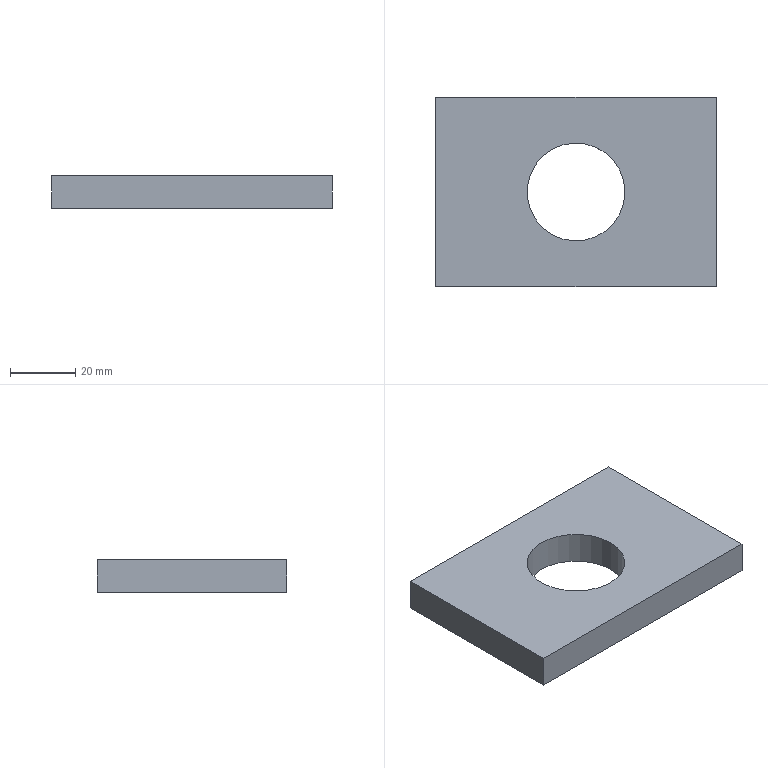Part | NX | features solid 2 | 1 solid | 7 faces | box 86 x 58 x 10 mm | volume 42811 mm3 | plane 6 | cylinder 1 | commonest cylinder face diameters 30 x1
STEP:
#1=CARTESIAN_POINT('',(534.,-7.,-170.));
#2=VERTEX_POINT('',#1);
#3=CARTESIAN_POINT('',(534.,-65.,-170.));
#4=VERTEX_POINT('',#3);
#5=CARTESIAN_POINT('',(534.,-12.,-170.));
#6=DIRECTION('',(0.,1.,0.));
#7=VECTOR('',#6,1000.);
#8=LINE('',#5,#7);
#9=EDGE_CURVE('',#2,#4,#8,.F.);
#10=ORIENTED_EDGE('',*,*,#9,.T.);
#11=CARTESIAN_POINT('',(534.,-65.,-180.));
#12=VERTEX_POINT('',#11);
#13=CARTESIAN_POINT('',(534.,-65.,-190.));
#14=DIRECTION('',(0.,0.,1.));
#15=VECTOR('',#14,1000.);
#16=LINE('',#13,#15);
#17=EDGE_CURVE('',#12,#4,#16,.T.);
#18=ORIENTED_EDGE('',*,*,#17,.F.);
#19=CARTESIAN_POINT('',(534.,-7.,-180.));
#20=VERTEX_POINT('',#19);
#21=CARTESIAN_POINT('',(534.,-12.,-180.));
#22=DIRECTION('',(0.,1.,0.));
#23=VECTOR('',#22,1000.);
#24=LINE('',#21,#23);
#25=EDGE_CURVE('',#20,#12,#24,.F.);
#26=ORIENTED_EDGE('',*,*,#25,.F.);
#27=CARTESIAN_POINT('',(534.,-7.,-190.));
#28=DIRECTION('',(0.,0.,1.));
#29=VECTOR('',#28,1000.);
#30=LINE('',#27,#29);
#31=EDGE_CURVE('',#20,#2,#30,.T.);
#32=ORIENTED_EDGE('',*,*,#31,.T.);
#33=EDGE_LOOP('',(#10,#18,#26,#32));
#34=FACE_BOUND('',#33,.T.);
#35=CARTESIAN_POINT('',(534.,-60.,-190.));
#36=DIRECTION('',(1.,0.,0.));
#37=DIRECTION('',(0.,0.,-1.));
#38=AXIS2_PLACEMENT_3D('',#35,#36,#37);
#39=PLANE('',#38);
#40=ADVANCED_FACE('',(#34),#39,.T.);
#41=CARTESIAN_POINT('',(448.,-65.,-170.));
#42=VERTEX_POINT('',#41);
#43=CARTESIAN_POINT('',(531.,-65.,-170.));
#44=DIRECTION('',(-1.,0.,0.));
#45=VECTOR('',#44,1000.);
#46=LINE('',#43,#45);
#47=EDGE_CURVE('',#42,#4,#46,.F.);
#48=ORIENTED_EDGE('',*,*,#47,.F.);
#49=CARTESIAN_POINT('',(448.,-65.,-180.));
#50=VERTEX_POINT('',#49);
#51=CARTESIAN_POINT('',(448.,-65.,-190.));
#52=DIRECTION('',(0.,0.,1.));
#53=VECTOR('',#52,1000.);
#54=LINE('',#51,#53);
#55=EDGE_CURVE('',#50,#42,#54,.T.);
#56=ORIENTED_EDGE('',*,*,#55,.F.);
#57=CARTESIAN_POINT('',(531.,-65.,-180.));
#58=DIRECTION('',(-1.,0.,0.));
#59=VECTOR('',#58,1000.);
#60=LINE('',#57,#59);
#61=EDGE_CURVE('',#50,#12,#60,.F.);
#62=ORIENTED_EDGE('',*,*,#61,.T.);
#63=ORIENTED_EDGE('',*,*,#17,.T.);
#64=EDGE_LOOP('',(#48,#56,#62,#63));
#65=FACE_BOUND('',#64,.T.);
#66=CARTESIAN_POINT('',(467.,-65.,-190.));
#67=DIRECTION('',(0.,1.,0.));
#68=DIRECTION('',(0.,0.,-1.));
#69=AXIS2_PLACEMENT_3D('',#66,#67,#68);
#70=PLANE('',#69);
#71=ADVANCED_FACE('',(#65),#70,.F.);
#72=CARTESIAN_POINT('',(448.,-7.,-170.));
#73=VERTEX_POINT('',#72);
#74=CARTESIAN_POINT('',(448.,-12.,-170.));
#75=DIRECTION('',(0.,1.,0.));
#76=VECTOR('',#75,1000.);
#77=LINE('',#74,#76);
#78=EDGE_CURVE('',#73,#42,#77,.F.);
#79=ORIENTED_EDGE('',*,*,#78,.F.);
#80=CARTESIAN_POINT('',(448.,-7.,-180.));
#81=VERTEX_POINT('',#80);
#82=CARTESIAN_POINT('',(448.,-7.,-190.));
#83=DIRECTION('',(0.,0.,1.));
#84=VECTOR('',#83,1000.);
#85=LINE('',#82,#84);
#86=EDGE_CURVE('',#81,#73,#85,.T.);
#87=ORIENTED_EDGE('',*,*,#86,.F.);
#88=CARTESIAN_POINT('',(448.,-12.,-180.));
#89=DIRECTION('',(0.,1.,0.));
#90=VECTOR('',#89,1000.);
#91=LINE('',#88,#90);
#92=EDGE_CURVE('',#81,#50,#91,.F.);
#93=ORIENTED_EDGE('',*,*,#92,.T.);
#94=ORIENTED_EDGE('',*,*,#55,.T.);
#95=EDGE_LOOP('',(#79,#87,#93,#94));
#96=FACE_BOUND('',#95,.T.);
#97=CARTESIAN_POINT('',(448.,-60.,-190.));
#98=DIRECTION('',(1.,0.,0.));
#99=DIRECTION('',(0.,0.,-1.));
#100=AXIS2_PLACEMENT_3D('',#97,#98,#99);
#101=PLANE('',#100);
#102=ADVANCED_FACE('',(#96),#101,.F.);
#103=CARTESIAN_POINT('',(531.,-7.,-170.));
#104=DIRECTION('',(-1.,0.,0.));
#105=VECTOR('',#104,1000.);
#106=LINE('',#103,#105);
#107=EDGE_CURVE('',#73,#2,#106,.F.);
#108=ORIENTED_EDGE('',*,*,#107,.T.);
#109=ORIENTED_EDGE('',*,*,#31,.F.);
#110=CARTESIAN_POINT('',(531.,-7.,-180.));
#111=DIRECTION('',(-1.,0.,0.));
#112=VECTOR('',#111,1000.);
#113=LINE('',#110,#112);
#114=EDGE_CURVE('',#81,#20,#113,.F.);
#115=ORIENTED_EDGE('',*,*,#114,.F.);
#116=ORIENTED_EDGE('',*,*,#86,.T.);
#117=EDGE_LOOP('',(#108,#109,#115,#116));
#118=FACE_BOUND('',#117,.T.);
#119=CARTESIAN_POINT('',(531.,-7.,-190.));
#120=DIRECTION('',(0.,1.,0.));
#121=DIRECTION('',(-1.,0.,0.));
#122=AXIS2_PLACEMENT_3D('',#119,#120,#121);
#123=PLANE('',#122);
#124=ADVANCED_FACE('',(#118),#123,.T.);
#125=CARTESIAN_POINT('',(506.,-36.,-180.));
#126=VERTEX_POINT('',#125);
#127=CARTESIAN_POINT('',(491.,-36.,-180.));
#128=DIRECTION('',(0.,0.,1.));
#129=DIRECTION('',(1.,0.,0.));
#130=AXIS2_PLACEMENT_3D('',#127,#128,#129);
#131=CIRCLE('',#130,15.);
#132=EDGE_CURVE('',#126,#126,#131,.T.);
#133=ORIENTED_EDGE('',*,*,#132,.T.);
#134=EDGE_LOOP('',(#133));
#135=FACE_BOUND('',#134,.T.);
#136=ORIENTED_EDGE('',*,*,#25,.T.);
#137=ORIENTED_EDGE('',*,*,#61,.F.);
#138=ORIENTED_EDGE('',*,*,#92,.F.);
#139=ORIENTED_EDGE('',*,*,#114,.T.);
#140=EDGE_LOOP('',(#136,#137,#138,#139));
#141=FACE_BOUND('',#140,.T.);
#142=CARTESIAN_POINT('',(531.,-12.,-180.));
#143=DIRECTION('',(0.,0.,1.));
#144=DIRECTION('',(1.,0.,0.));
#145=AXIS2_PLACEMENT_3D('',#142,#143,#144);
#146=PLANE('',#145);
#147=ADVANCED_FACE('',(#135,#141),#146,.F.);
#148=CARTESIAN_POINT('',(506.,-36.,-170.));
#149=VERTEX_POINT('',#148);
#150=CARTESIAN_POINT('',(491.,-36.,-170.));
#151=DIRECTION('',(0.,0.,1.));
#152=DIRECTION('',(1.,0.,0.));
#153=AXIS2_PLACEMENT_3D('',#150,#151,#152);
#154=CIRCLE('',#153,15.);
#155=EDGE_CURVE('',#149,#149,#154,.T.);
#156=ORIENTED_EDGE('',*,*,#155,.F.);
#157=EDGE_LOOP('',(#156));
#158=FACE_BOUND('',#157,.T.);
#159=ORIENTED_EDGE('',*,*,#9,.F.);
#160=ORIENTED_EDGE('',*,*,#107,.F.);
#161=ORIENTED_EDGE('',*,*,#78,.T.);
#162=ORIENTED_EDGE('',*,*,#47,.T.);
#163=EDGE_LOOP('',(#159,#160,#161,#162));
#164=FACE_BOUND('',#163,.T.);
#165=CARTESIAN_POINT('',(531.,-12.,-170.));
#166=DIRECTION('',(0.,0.,1.));
#167=DIRECTION('',(1.,0.,0.));
#168=AXIS2_PLACEMENT_3D('',#165,#166,#167);
#169=PLANE('',#168);
#170=ADVANCED_FACE('',(#158,#164),#169,.T.);
#171=ORIENTED_EDGE('',*,*,#155,.T.);
#172=EDGE_LOOP('',(#171));
#173=FACE_BOUND('',#172,.T.);
#174=ORIENTED_EDGE('',*,*,#132,.F.);
#175=EDGE_LOOP('',(#174));
#176=FACE_BOUND('',#175,.T.);
#177=CARTESIAN_POINT('',(491.,-36.,-176.));
#178=DIRECTION('',(0.,0.,1.));
#179=DIRECTION('',(1.,0.,0.));
#180=AXIS2_PLACEMENT_3D('',#177,#178,#179);
#181=CYLINDRICAL_SURFACE('',#180,15.);
#182=ADVANCED_FACE('',(#173,#176),#181,.F.);
#183=CLOSED_SHELL('',(#40,#71,#102,#124,#147,#170,#182));
#184=MANIFOLD_SOLID_BREP('',#183);
#185=(LENGTH_UNIT()NAMED_UNIT(*)SI_UNIT(.MILLI.,.METRE.));
#186=UNCERTAINTY_MEASURE_WITH_UNIT(LENGTH_MEASURE(0.00001),#185,'','');
#187=(NAMED_UNIT(*)PLANE_ANGLE_UNIT()SI_UNIT($,.RADIAN.));
#188=(NAMED_UNIT(*)SI_UNIT($,.STERADIAN.)SOLID_ANGLE_UNIT());
#189=(GEOMETRIC_REPRESENTATION_CONTEXT(3)GLOBAL_UNCERTAINTY_ASSIGNED_CONTEXT((#186))GLOBAL_UNIT_ASSIGNED_CONTEXT((#185,#187,#188))REPRESENTATION_CONTEXT('',''));
#190=ADVANCED_BREP_SHAPE_REPRESENTATION('',(#184),#189);